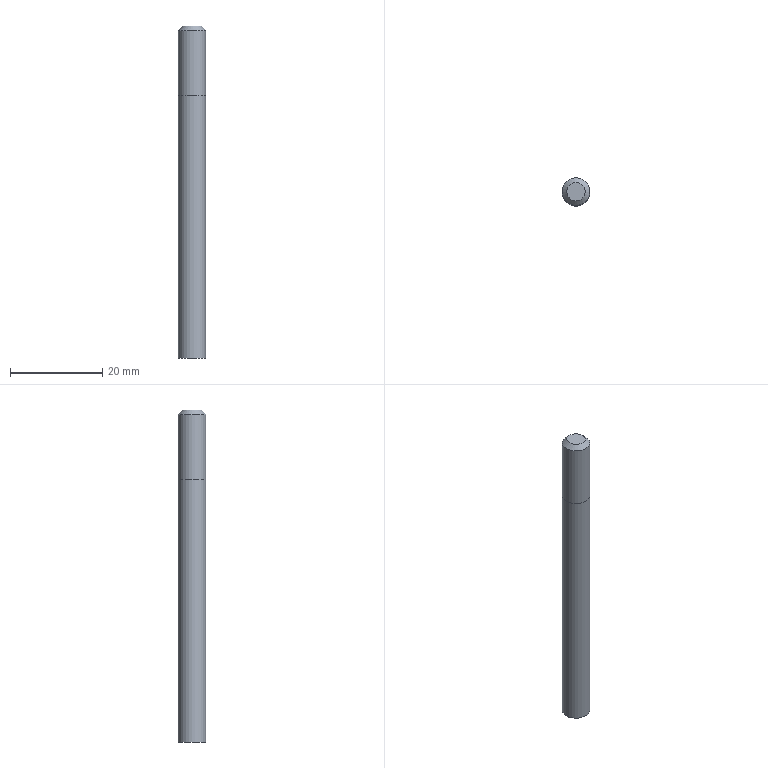Part | NX | features BREP 1, DATUM_CSYS 1 | 1 solid | 5 faces | box 6 x 6 x 72 mm | volume 2027 mm3 | plane 2 | cylinder 2 | cone 1 | commonest cylinder face diameters 6 x2
STEP:
#1=CARTESIAN_POINT('',(3.,0.,0.));
#2=VERTEX_POINT('',#1);
#3=CARTESIAN_POINT('',(0.,0.,0.));
#4=DIRECTION('',(0.,0.,1.));
#5=DIRECTION('',(1.,0.,0.));
#6=AXIS2_PLACEMENT_3D('',#3,#4,#5);
#7=CIRCLE('',#6,3.);
#8=EDGE_CURVE('',#2,#2,#7,.T.);
#9=ORIENTED_EDGE('',*,*,#8,.F.);
#10=EDGE_LOOP('',(#9));
#11=FACE_BOUND('',#10,.T.);
#12=CARTESIAN_POINT('',(0.,0.,0.));
#13=DIRECTION('',(0.,0.,1.));
#14=DIRECTION('',(-1.,0.,0.));
#15=AXIS2_PLACEMENT_3D('',#12,#13,#14);
#16=PLANE('',#15);
#17=ADVANCED_FACE('',(#11),#16,.F.);
#18=CARTESIAN_POINT('',(2.,0.,72.));
#19=VERTEX_POINT('',#18);
#20=CARTESIAN_POINT('',(0.,0.,72.));
#21=DIRECTION('',(0.,0.,-1.));
#22=DIRECTION('',(1.,0.,0.));
#23=AXIS2_PLACEMENT_3D('',#20,#21,#22);
#24=CIRCLE('',#23,2.);
#25=EDGE_CURVE('',#19,#19,#24,.T.);
#26=ORIENTED_EDGE('',*,*,#25,.F.);
#27=EDGE_LOOP('',(#26));
#28=FACE_BOUND('',#27,.T.);
#29=CARTESIAN_POINT('',(0.,0.,72.));
#30=DIRECTION('',(0.,0.,1.));
#31=DIRECTION('',(-1.,0.,0.));
#32=AXIS2_PLACEMENT_3D('',#29,#30,#31);
#33=PLANE('',#32);
#34=ADVANCED_FACE('',(#28),#33,.T.);
#35=ORIENTED_EDGE('',*,*,#8,.T.);
#36=CARTESIAN_POINT('',(3.,0.,57.));
#37=VERTEX_POINT('',#36);
#38=CARTESIAN_POINT('',(3.,0.,0.));
#39=DIRECTION('',(0.,0.,1.));
#40=VECTOR('',#39,1000.);
#41=LINE('',#38,#40);
#42=EDGE_CURVE('',#2,#37,#41,.T.);
#43=ORIENTED_EDGE('',*,*,#42,.T.);
#44=CARTESIAN_POINT('',(0.,0.,57.));
#45=DIRECTION('',(0.,0.,1.));
#46=DIRECTION('',(1.,0.,0.));
#47=AXIS2_PLACEMENT_3D('',#44,#45,#46);
#48=CIRCLE('',#47,3.);
#49=EDGE_CURVE('',#37,#37,#48,.T.);
#50=ORIENTED_EDGE('',*,*,#49,.F.);
#51=ORIENTED_EDGE('',*,*,#42,.F.);
#52=EDGE_LOOP('',(#35,#43,#50,#51));
#53=FACE_BOUND('',#52,.T.);
#54=CARTESIAN_POINT('',(0.,0.,0.));
#55=DIRECTION('',(0.,0.,1.));
#56=DIRECTION('',(-1.,0.,0.));
#57=AXIS2_PLACEMENT_3D('',#54,#55,#56);
#58=CYLINDRICAL_SURFACE('',#57,3.);
#59=ADVANCED_FACE('',(#53),#58,.T.);
#60=ORIENTED_EDGE('',*,*,#49,.T.);
#61=CARTESIAN_POINT('',(3.,0.,71.));
#62=VERTEX_POINT('',#61);
#63=CARTESIAN_POINT('',(3.,0.,57.));
#64=DIRECTION('',(0.,0.,1.));
#65=VECTOR('',#64,1000.);
#66=LINE('',#63,#65);
#67=EDGE_CURVE('',#37,#62,#66,.T.);
#68=ORIENTED_EDGE('',*,*,#67,.T.);
#69=CARTESIAN_POINT('',(0.,0.,71.));
#70=DIRECTION('',(0.,0.,-1.));
#71=DIRECTION('',(1.,0.,0.));
#72=AXIS2_PLACEMENT_3D('',#69,#70,#71);
#73=CIRCLE('',#72,3.);
#74=EDGE_CURVE('',#62,#62,#73,.T.);
#75=ORIENTED_EDGE('',*,*,#74,.T.);
#76=ORIENTED_EDGE('',*,*,#67,.F.);
#77=EDGE_LOOP('',(#60,#68,#75,#76));
#78=FACE_BOUND('',#77,.T.);
#79=CARTESIAN_POINT('',(0.,0.,57.));
#80=DIRECTION('',(0.,0.,1.));
#81=DIRECTION('',(-1.,0.,0.));
#82=AXIS2_PLACEMENT_3D('',#79,#80,#81);
#83=CYLINDRICAL_SURFACE('',#82,3.);
#84=ADVANCED_FACE('',(#78),#83,.T.);
#85=CARTESIAN_POINT('',(2.,0.,72.));
#86=DIRECTION('',(0.7071,0.,-0.7071));
#87=VECTOR('',#86,1000.);
#88=LINE('',#85,#87);
#89=EDGE_CURVE('',#19,#62,#88,.T.);
#90=ORIENTED_EDGE('',*,*,#89,.T.);
#91=ORIENTED_EDGE('',*,*,#74,.F.);
#92=ORIENTED_EDGE('',*,*,#89,.F.);
#93=ORIENTED_EDGE('',*,*,#25,.T.);
#94=EDGE_LOOP('',(#90,#91,#92,#93));
#95=FACE_BOUND('',#94,.T.);
#96=CARTESIAN_POINT('',(0.,0.,72.));
#97=DIRECTION('',(0.,0.,-1.));
#98=DIRECTION('',(-1.,0.,0.));
#99=AXIS2_PLACEMENT_3D('',#96,#97,#98);
#100=CONICAL_SURFACE('',#99,2.,0.7854);
#101=ADVANCED_FACE('',(#95),#100,.T.);
#102=CLOSED_SHELL('',(#17,#34,#59,#84,#101));
#103=MANIFOLD_SOLID_BREP('',#102);
#104=(LENGTH_UNIT()NAMED_UNIT(*)SI_UNIT(.MILLI.,.METRE.));
#105=UNCERTAINTY_MEASURE_WITH_UNIT(LENGTH_MEASURE(0.00001),#104,'','');
#106=(NAMED_UNIT(*)PLANE_ANGLE_UNIT()SI_UNIT($,.RADIAN.));
#107=(NAMED_UNIT(*)SI_UNIT($,.STERADIAN.)SOLID_ANGLE_UNIT());
#108=(GEOMETRIC_REPRESENTATION_CONTEXT(3)GLOBAL_UNCERTAINTY_ASSIGNED_CONTEXT((#105))GLOBAL_UNIT_ASSIGNED_CONTEXT((#104,#106,#107))REPRESENTATION_CONTEXT('',''));
#109=ADVANCED_BREP_SHAPE_REPRESENTATION('',(#103),#108);